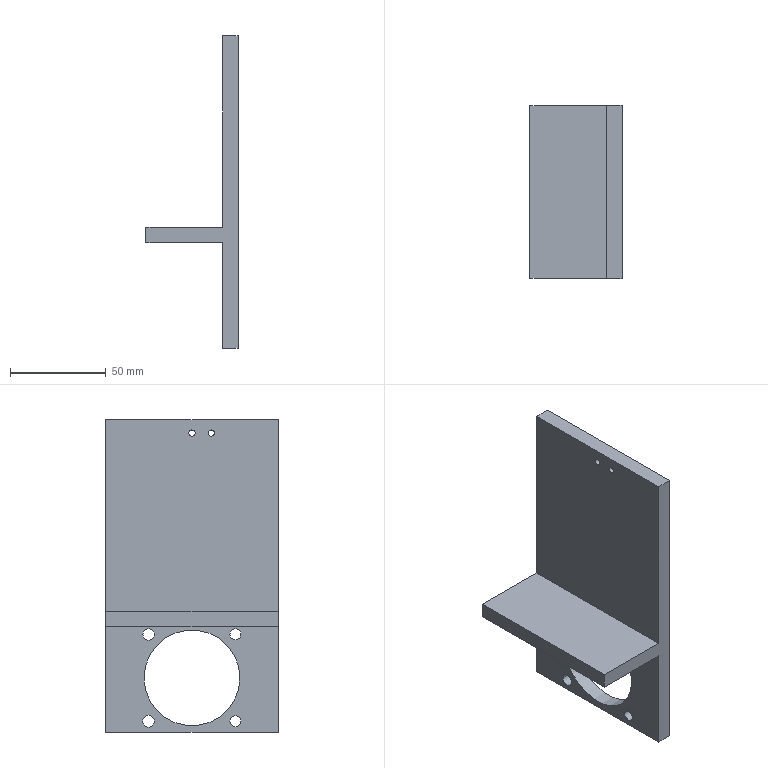Part | SolidWorks | features ICE 3, Cut 2, Extrusion 1, HoleWzd 1 | 1 solid | 24 faces | box 48 x 90 x 163 mm | volume 129456 mm3 | cylinder 14 | plane 10 | commonest cylinder face diameters 3.3 x4 5.748 x2 5.749 x2 5.963 x2 6.073 x2 49.982 x2
STEP:
#1=CARTESIAN_POINT('',(-62.,0.,99.35));
#2=VERTEX_POINT('',#1);
#3=CARTESIAN_POINT('',(-62.,0.,102.65));
#4=VERTEX_POINT('',#3);
#5=CARTESIAN_POINT('',(-62.,0.,101.));
#6=DIRECTION('',(-1.,0.,0.));
#7=DIRECTION('',(0.,-1.,0.));
#8=AXIS2_PLACEMENT_3D('',#5,#6,#7);
#9=CIRCLE('',#8,1.65);
#10=EDGE_CURVE('',#2,#4,#9,.T.);
#11=ORIENTED_EDGE('',*,*,#10,.F.);
#12=CARTESIAN_POINT('',(-70.,0.,99.35));
#13=VERTEX_POINT('',#12);
#14=CARTESIAN_POINT('',(-70.,0.,99.35));
#15=DIRECTION('',(-1.,0.,0.));
#16=VECTOR('',#15,1000.);
#17=LINE('',#14,#16);
#18=EDGE_CURVE('',#2,#13,#17,.T.);
#19=ORIENTED_EDGE('',*,*,#18,.T.);
#20=CARTESIAN_POINT('',(-70.,0.,102.65));
#21=VERTEX_POINT('',#20);
#22=CARTESIAN_POINT('',(-70.,0.,101.));
#23=DIRECTION('',(-1.,0.,0.));
#24=DIRECTION('',(0.,0.,1.));
#25=AXIS2_PLACEMENT_3D('',#22,#23,#24);
#26=CIRCLE('',#25,1.65);
#27=EDGE_CURVE('',#13,#21,#26,.T.);
#28=ORIENTED_EDGE('',*,*,#27,.T.);
#29=CARTESIAN_POINT('',(-70.,0.,102.65));
#30=DIRECTION('',(-1.,0.,0.));
#31=VECTOR('',#30,1000.);
#32=LINE('',#29,#31);
#33=EDGE_CURVE('',#4,#21,#32,.T.);
#34=ORIENTED_EDGE('',*,*,#33,.F.);
#35=EDGE_LOOP('',(#11,#19,#28,#34));
#36=FACE_OUTER_BOUND('',#35,.T.);
#37=CARTESIAN_POINT('',(-70.,0.,101.));
#38=DIRECTION('',(-1.,0.,0.));
#39=DIRECTION('',(0.,0.,1.));
#40=AXIS2_PLACEMENT_3D('',#37,#38,#39);
#41=CYLINDRICAL_SURFACE('',#40,1.65);
#42=ADVANCED_FACE('',(#36),#41,.F.);
#43=CARTESIAN_POINT('',(-62.,-10.,99.35));
#44=VERTEX_POINT('',#43);
#45=CARTESIAN_POINT('',(-62.,-10.,102.65));
#46=VERTEX_POINT('',#45);
#47=CARTESIAN_POINT('',(-62.,-10.,101.));
#48=DIRECTION('',(-1.,0.,0.));
#49=DIRECTION('',(0.,-1.,0.));
#50=AXIS2_PLACEMENT_3D('',#47,#48,#49);
#51=CIRCLE('',#50,1.65);
#52=EDGE_CURVE('',#44,#46,#51,.T.);
#53=ORIENTED_EDGE('',*,*,#52,.F.);
#54=CARTESIAN_POINT('',(-70.,-10.,99.35));
#55=VERTEX_POINT('',#54);
#56=CARTESIAN_POINT('',(-70.,-10.,99.35));
#57=DIRECTION('',(-1.,0.,0.));
#58=VECTOR('',#57,1000.);
#59=LINE('',#56,#58);
#60=EDGE_CURVE('',#44,#55,#59,.T.);
#61=ORIENTED_EDGE('',*,*,#60,.T.);
#62=CARTESIAN_POINT('',(-70.,-10.,102.65));
#63=VERTEX_POINT('',#62);
#64=CARTESIAN_POINT('',(-70.,-10.,101.));
#65=DIRECTION('',(-1.,0.,0.));
#66=DIRECTION('',(0.,0.,1.));
#67=AXIS2_PLACEMENT_3D('',#64,#65,#66);
#68=CIRCLE('',#67,1.65);
#69=EDGE_CURVE('',#55,#63,#68,.T.);
#70=ORIENTED_EDGE('',*,*,#69,.T.);
#71=CARTESIAN_POINT('',(-70.,-10.,102.65));
#72=DIRECTION('',(-1.,0.,0.));
#73=VECTOR('',#72,1000.);
#74=LINE('',#71,#73);
#75=EDGE_CURVE('',#46,#63,#74,.T.);
#76=ORIENTED_EDGE('',*,*,#75,.F.);
#77=EDGE_LOOP('',(#53,#61,#70,#76));
#78=FACE_OUTER_BOUND('',#77,.T.);
#79=CARTESIAN_POINT('',(-70.,-10.,101.));
#80=DIRECTION('',(-1.,0.,0.));
#81=DIRECTION('',(0.,0.,1.));
#82=AXIS2_PLACEMENT_3D('',#79,#80,#81);
#83=CYLINDRICAL_SURFACE('',#82,1.65);
#84=ADVANCED_FACE('',(#78),#83,.F.);
#85=CARTESIAN_POINT('',(-62.,25.609,-3.973));
#86=VERTEX_POINT('',#85);
#87=CARTESIAN_POINT('',(-62.,19.646,-3.973));
#88=VERTEX_POINT('',#87);
#89=CARTESIAN_POINT('',(-62.,22.627,-3.973));
#90=DIRECTION('',(-1.,0.,0.));
#91=DIRECTION('',(0.,-1.,0.));
#92=AXIS2_PLACEMENT_3D('',#89,#90,#91);
#93=CIRCLE('',#92,2.981);
#94=EDGE_CURVE('',#86,#88,#93,.T.);
#95=ORIENTED_EDGE('',*,*,#94,.F.);
#96=CARTESIAN_POINT('',(-70.,25.609,-3.973));
#97=VERTEX_POINT('',#96);
#98=CARTESIAN_POINT('',(-35.,25.609,-3.973));
#99=DIRECTION('',(-1.,0.,0.));
#100=VECTOR('',#99,1000.);
#101=LINE('',#98,#100);
#102=EDGE_CURVE('',#86,#97,#101,.T.);
#103=ORIENTED_EDGE('',*,*,#102,.T.);
#104=CARTESIAN_POINT('',(-70.,19.646,-3.973));
#105=VERTEX_POINT('',#104);
#106=CARTESIAN_POINT('',(-70.,22.627,-3.973));
#107=DIRECTION('',(-1.,0.,0.));
#108=DIRECTION('',(0.,-1.,0.));
#109=AXIS2_PLACEMENT_3D('',#106,#107,#108);
#110=CIRCLE('',#109,2.981);
#111=EDGE_CURVE('',#97,#105,#110,.T.);
#112=ORIENTED_EDGE('',*,*,#111,.T.);
#113=CARTESIAN_POINT('',(-35.,19.646,-3.973));
#114=DIRECTION('',(-1.,0.,0.));
#115=VECTOR('',#114,1000.);
#116=LINE('',#113,#115);
#117=EDGE_CURVE('',#88,#105,#116,.T.);
#118=ORIENTED_EDGE('',*,*,#117,.F.);
#119=EDGE_LOOP('',(#95,#103,#112,#118));
#120=FACE_OUTER_BOUND('',#119,.T.);
#121=CARTESIAN_POINT('',(-35.,22.627,-3.973));
#122=DIRECTION('',(-1.,0.,0.));
#123=DIRECTION('',(0.,-1.,0.));
#124=AXIS2_PLACEMENT_3D('',#121,#122,#123);
#125=CYLINDRICAL_SURFACE('',#124,2.981);
#126=ADVANCED_FACE('',(#120),#125,.F.);
#127=CARTESIAN_POINT('',(-62.,-19.753,-3.973));
#128=VERTEX_POINT('',#127);
#129=CARTESIAN_POINT('',(-62.,-25.502,-3.973));
#130=VERTEX_POINT('',#129);
#131=CARTESIAN_POINT('',(-62.,-22.627,-3.973));
#132=DIRECTION('',(-1.,0.,0.));
#133=DIRECTION('',(0.,-1.,0.));
#134=AXIS2_PLACEMENT_3D('',#131,#132,#133);
#135=CIRCLE('',#134,2.874);
#136=EDGE_CURVE('',#128,#130,#135,.T.);
#137=ORIENTED_EDGE('',*,*,#136,.F.);
#138=CARTESIAN_POINT('',(-70.,-19.753,-3.973));
#139=VERTEX_POINT('',#138);
#140=CARTESIAN_POINT('',(-35.,-19.753,-3.973));
#141=DIRECTION('',(-1.,0.,0.));
#142=VECTOR('',#141,1000.);
#143=LINE('',#140,#142);
#144=EDGE_CURVE('',#128,#139,#143,.T.);
#145=ORIENTED_EDGE('',*,*,#144,.T.);
#146=CARTESIAN_POINT('',(-70.,-25.502,-3.973));
#147=VERTEX_POINT('',#146);
#148=CARTESIAN_POINT('',(-70.,-22.627,-3.973));
#149=DIRECTION('',(-1.,0.,0.));
#150=DIRECTION('',(0.,-1.,0.));
#151=AXIS2_PLACEMENT_3D('',#148,#149,#150);
#152=CIRCLE('',#151,2.874);
#153=EDGE_CURVE('',#139,#147,#152,.T.);
#154=ORIENTED_EDGE('',*,*,#153,.T.);
#155=CARTESIAN_POINT('',(-35.,-25.502,-3.973));
#156=DIRECTION('',(-1.,0.,0.));
#157=VECTOR('',#156,1000.);
#158=LINE('',#155,#157);
#159=EDGE_CURVE('',#130,#147,#158,.T.);
#160=ORIENTED_EDGE('',*,*,#159,.F.);
#161=EDGE_LOOP('',(#137,#145,#154,#160));
#162=FACE_OUTER_BOUND('',#161,.T.);
#163=CARTESIAN_POINT('',(-35.,-22.627,-3.973));
#164=DIRECTION('',(-1.,0.,0.));
#165=DIRECTION('',(0.,-1.,0.));
#166=AXIS2_PLACEMENT_3D('',#163,#164,#165);
#167=CYLINDRICAL_SURFACE('',#166,2.874);
#168=ADVANCED_FACE('',(#162),#167,.F.);
#169=CARTESIAN_POINT('',(-62.,-19.754,-49.227));
#170=VERTEX_POINT('',#169);
#171=CARTESIAN_POINT('',(-62.,-25.501,-49.227));
#172=VERTEX_POINT('',#171);
#173=CARTESIAN_POINT('',(-62.,-22.627,-49.227));
#174=DIRECTION('',(-1.,0.,0.));
#175=DIRECTION('',(0.,-1.,0.));
#176=AXIS2_PLACEMENT_3D('',#173,#174,#175);
#177=CIRCLE('',#176,2.874);
#178=EDGE_CURVE('',#170,#172,#177,.T.);
#179=ORIENTED_EDGE('',*,*,#178,.F.);
#180=CARTESIAN_POINT('',(-70.,-19.754,-49.227));
#181=VERTEX_POINT('',#180);
#182=CARTESIAN_POINT('',(-35.,-19.754,-49.227));
#183=DIRECTION('',(-1.,0.,0.));
#184=VECTOR('',#183,1000.);
#185=LINE('',#182,#184);
#186=EDGE_CURVE('',#170,#181,#185,.T.);
#187=ORIENTED_EDGE('',*,*,#186,.T.);
#188=CARTESIAN_POINT('',(-70.,-25.501,-49.227));
#189=VERTEX_POINT('',#188);
#190=CARTESIAN_POINT('',(-70.,-22.627,-49.227));
#191=DIRECTION('',(-1.,0.,0.));
#192=DIRECTION('',(0.,-1.,0.));
#193=AXIS2_PLACEMENT_3D('',#190,#191,#192);
#194=CIRCLE('',#193,2.874);
#195=EDGE_CURVE('',#181,#189,#194,.T.);
#196=ORIENTED_EDGE('',*,*,#195,.T.);
#197=CARTESIAN_POINT('',(-35.,-25.501,-49.227));
#198=DIRECTION('',(-1.,0.,0.));
#199=VECTOR('',#198,1000.);
#200=LINE('',#197,#199);
#201=EDGE_CURVE('',#172,#189,#200,.T.);
#202=ORIENTED_EDGE('',*,*,#201,.F.);
#203=EDGE_LOOP('',(#179,#187,#196,#202));
#204=FACE_OUTER_BOUND('',#203,.T.);
#205=CARTESIAN_POINT('',(-35.,-22.627,-49.227));
#206=DIRECTION('',(-1.,0.,0.));
#207=DIRECTION('',(0.,-1.,0.));
#208=AXIS2_PLACEMENT_3D('',#205,#206,#207);
#209=CYLINDRICAL_SURFACE('',#208,2.874);
#210=ADVANCED_FACE('',(#204),#209,.F.);
#211=CARTESIAN_POINT('',(-62.,25.664,-49.227));
#212=VERTEX_POINT('',#211);
#213=CARTESIAN_POINT('',(-62.,19.591,-49.227));
#214=VERTEX_POINT('',#213);
#215=CARTESIAN_POINT('',(-62.,22.627,-49.227));
#216=DIRECTION('',(-1.,0.,0.));
#217=DIRECTION('',(0.,-1.,0.));
#218=AXIS2_PLACEMENT_3D('',#215,#216,#217);
#219=CIRCLE('',#218,3.036);
#220=EDGE_CURVE('',#212,#214,#219,.T.);
#221=ORIENTED_EDGE('',*,*,#220,.F.);
#222=CARTESIAN_POINT('',(-70.,25.664,-49.227));
#223=VERTEX_POINT('',#222);
#224=CARTESIAN_POINT('',(-35.,25.664,-49.227));
#225=DIRECTION('',(-1.,0.,0.));
#226=VECTOR('',#225,1000.);
#227=LINE('',#224,#226);
#228=EDGE_CURVE('',#212,#223,#227,.T.);
#229=ORIENTED_EDGE('',*,*,#228,.T.);
#230=CARTESIAN_POINT('',(-70.,19.591,-49.227));
#231=VERTEX_POINT('',#230);
#232=CARTESIAN_POINT('',(-70.,22.627,-49.227));
#233=DIRECTION('',(-1.,0.,0.));
#234=DIRECTION('',(0.,-1.,0.));
#235=AXIS2_PLACEMENT_3D('',#232,#233,#234);
#236=CIRCLE('',#235,3.036);
#237=EDGE_CURVE('',#223,#231,#236,.T.);
#238=ORIENTED_EDGE('',*,*,#237,.T.);
#239=CARTESIAN_POINT('',(-35.,19.591,-49.227));
#240=DIRECTION('',(-1.,0.,0.));
#241=VECTOR('',#240,1000.);
#242=LINE('',#239,#241);
#243=EDGE_CURVE('',#214,#231,#242,.T.);
#244=ORIENTED_EDGE('',*,*,#243,.F.);
#245=EDGE_LOOP('',(#221,#229,#238,#244));
#246=FACE_OUTER_BOUND('',#245,.T.);
#247=CARTESIAN_POINT('',(-35.,22.627,-49.227));
#248=DIRECTION('',(-1.,0.,0.));
#249=DIRECTION('',(0.,-1.,0.));
#250=AXIS2_PLACEMENT_3D('',#247,#248,#249);
#251=CYLINDRICAL_SURFACE('',#250,3.036);
#252=ADVANCED_FACE('',(#246),#251,.F.);
#253=CARTESIAN_POINT('',(-62.,25.,-26.6));
#254=VERTEX_POINT('',#253);
#255=CARTESIAN_POINT('',(-62.,-24.982,-26.6));
#256=VERTEX_POINT('',#255);
#257=CARTESIAN_POINT('',(-62.,0.009138,-26.6));
#258=DIRECTION('',(-1.,0.,0.));
#259=DIRECTION('',(0.,-1.,0.));
#260=AXIS2_PLACEMENT_3D('',#257,#258,#259);
#261=CIRCLE('',#260,24.991);
#262=EDGE_CURVE('',#254,#256,#261,.T.);
#263=ORIENTED_EDGE('',*,*,#262,.F.);
#264=CARTESIAN_POINT('',(-70.,25.,-26.6));
#265=VERTEX_POINT('',#264);
#266=CARTESIAN_POINT('',(-35.,25.,-26.6));
#267=DIRECTION('',(-1.,0.,0.));
#268=VECTOR('',#267,1000.);
#269=LINE('',#266,#268);
#270=EDGE_CURVE('',#254,#265,#269,.T.);
#271=ORIENTED_EDGE('',*,*,#270,.T.);
#272=CARTESIAN_POINT('',(-70.,-24.982,-26.6));
#273=VERTEX_POINT('',#272);
#274=CARTESIAN_POINT('',(-70.,0.009138,-26.6));
#275=DIRECTION('',(-1.,0.,0.));
#276=DIRECTION('',(0.,-1.,0.));
#277=AXIS2_PLACEMENT_3D('',#274,#275,#276);
#278=CIRCLE('',#277,24.991);
#279=EDGE_CURVE('',#265,#273,#278,.T.);
#280=ORIENTED_EDGE('',*,*,#279,.T.);
#281=CARTESIAN_POINT('',(-35.,-24.982,-26.6));
#282=DIRECTION('',(-1.,0.,0.));
#283=VECTOR('',#282,1000.);
#284=LINE('',#281,#283);
#285=EDGE_CURVE('',#256,#273,#284,.T.);
#286=ORIENTED_EDGE('',*,*,#285,.F.);
#287=EDGE_LOOP('',(#263,#271,#280,#286));
#288=FACE_OUTER_BOUND('',#287,.T.);
#289=CARTESIAN_POINT('',(-35.,0.009138,-26.6));
#290=DIRECTION('',(-1.,0.,0.));
#291=DIRECTION('',(0.,-1.,0.));
#292=AXIS2_PLACEMENT_3D('',#289,#290,#291);
#293=CYLINDRICAL_SURFACE('',#292,24.991);
#294=ADVANCED_FACE('',(#288),#293,.F.);
#295=CARTESIAN_POINT('',(-70.,-45.,0.));
#296=VERTEX_POINT('',#295);
#297=CARTESIAN_POINT('',(-70.,45.,0.));
#298=VERTEX_POINT('',#297);
#299=CARTESIAN_POINT('',(-70.,-45.,0.));
#300=DIRECTION('',(0.,1.,0.));
#301=VECTOR('',#300,1000.);
#302=LINE('',#299,#301);
#303=EDGE_CURVE('',#296,#298,#302,.T.);
#304=ORIENTED_EDGE('',*,*,#303,.F.);
#305=CARTESIAN_POINT('',(-110.,-45.,0.));
#306=VERTEX_POINT('',#305);
#307=CARTESIAN_POINT('',(-60.,-45.,0.));
#308=DIRECTION('',(1.,0.,0.));
#309=VECTOR('',#308,1000.);
#310=LINE('',#307,#309);
#311=EDGE_CURVE('',#306,#296,#310,.T.);
#312=ORIENTED_EDGE('',*,*,#311,.F.);
#313=CARTESIAN_POINT('',(-110.,45.,0.));
#314=VERTEX_POINT('',#313);
#315=CARTESIAN_POINT('',(-110.,45.,0.));
#316=DIRECTION('',(0.,-1.,0.));
#317=VECTOR('',#316,1000.);
#318=LINE('',#315,#317);
#319=EDGE_CURVE('',#314,#306,#318,.T.);
#320=ORIENTED_EDGE('',*,*,#319,.F.);
#321=CARTESIAN_POINT('',(-60.,45.,0.));
#322=DIRECTION('',(-1.,0.,0.));
#323=VECTOR('',#322,1000.);
#324=LINE('',#321,#323);
#325=EDGE_CURVE('',#298,#314,#324,.T.);
#326=ORIENTED_EDGE('',*,*,#325,.F.);
#327=EDGE_LOOP('',(#304,#312,#320,#326));
#328=FACE_OUTER_BOUND('',#327,.T.);
#329=CARTESIAN_POINT('',(0.,0.,0.));
#330=DIRECTION('',(0.,0.,1.));
#331=DIRECTION('',(1.,0.,0.));
#332=AXIS2_PLACEMENT_3D('',#329,#330,#331);
#333=PLANE('',#332);
#334=ADVANCED_FACE('',(#328),#333,.F.);
#335=CARTESIAN_POINT('',(-70.,45.,8.));
#336=VERTEX_POINT('',#335);
#337=CARTESIAN_POINT('',(-70.,-45.,8.));
#338=VERTEX_POINT('',#337);
#339=CARTESIAN_POINT('',(-70.,45.,8.));
#340=DIRECTION('',(0.,-1.,0.));
#341=VECTOR('',#340,1000.);
#342=LINE('',#339,#341);
#343=EDGE_CURVE('',#336,#338,#342,.T.);
#344=ORIENTED_EDGE('',*,*,#343,.F.);
#345=CARTESIAN_POINT('',(-110.,45.,8.));
#346=VERTEX_POINT('',#345);
#347=CARTESIAN_POINT('',(-60.,45.,8.));
#348=DIRECTION('',(-1.,0.,0.));
#349=VECTOR('',#348,1000.);
#350=LINE('',#347,#349);
#351=EDGE_CURVE('',#336,#346,#350,.T.);
#352=ORIENTED_EDGE('',*,*,#351,.T.);
#353=CARTESIAN_POINT('',(-110.,-45.,8.));
#354=VERTEX_POINT('',#353);
#355=CARTESIAN_POINT('',(-110.,-45.,8.));
#356=DIRECTION('',(0.,1.,0.));
#357=VECTOR('',#356,1000.);
#358=LINE('',#355,#357);
#359=EDGE_CURVE('',#354,#346,#358,.T.);
#360=ORIENTED_EDGE('',*,*,#359,.F.);
#361=CARTESIAN_POINT('',(-60.,-45.,8.));
#362=DIRECTION('',(1.,0.,0.));
#363=VECTOR('',#362,1000.);
#364=LINE('',#361,#363);
#365=EDGE_CURVE('',#354,#338,#364,.T.);
#366=ORIENTED_EDGE('',*,*,#365,.T.);
#367=EDGE_LOOP('',(#344,#352,#360,#366));
#368=FACE_OUTER_BOUND('',#367,.T.);
#369=CARTESIAN_POINT('',(0.,0.,8.));
#370=DIRECTION('',(0.,0.,1.));
#371=DIRECTION('',(1.,0.,0.));
#372=AXIS2_PLACEMENT_3D('',#369,#370,#371);
#373=PLANE('',#372);
#374=ADVANCED_FACE('',(#368),#373,.T.);
#375=CARTESIAN_POINT('',(-62.,45.,108.));
#376=VERTEX_POINT('',#375);
#377=CARTESIAN_POINT('',(-62.,45.,-55.));
#378=VERTEX_POINT('',#377);
#379=CARTESIAN_POINT('',(-62.,45.,108.));
#380=DIRECTION('',(0.,0.,-1.));
#381=VECTOR('',#380,1000.);
#382=LINE('',#379,#381);
#383=EDGE_CURVE('',#376,#378,#382,.T.);
#384=ORIENTED_EDGE('',*,*,#383,.T.);
#385=CARTESIAN_POINT('',(-70.,45.,-55.));
#386=VERTEX_POINT('',#385);
#387=CARTESIAN_POINT('',(-70.,45.,-55.));
#388=DIRECTION('',(1.,0.,0.));
#389=VECTOR('',#388,1000.);
#390=LINE('',#387,#389);
#391=EDGE_CURVE('',#386,#378,#390,.T.);
#392=ORIENTED_EDGE('',*,*,#391,.F.);
#393=CARTESIAN_POINT('',(-70.,45.,-55.));
#394=DIRECTION('',(0.,0.,1.));
#395=VECTOR('',#394,1000.);
#396=LINE('',#393,#395);
#397=EDGE_CURVE('',#386,#298,#396,.T.);
#398=ORIENTED_EDGE('',*,*,#397,.T.);
#399=ORIENTED_EDGE('',*,*,#325,.T.);
#400=CARTESIAN_POINT('',(-110.,45.,8.));
#401=DIRECTION('',(0.,0.,-1.));
#402=VECTOR('',#401,1000.);
#403=LINE('',#400,#402);
#404=EDGE_CURVE('',#346,#314,#403,.T.);
#405=ORIENTED_EDGE('',*,*,#404,.F.);
#406=ORIENTED_EDGE('',*,*,#351,.F.);
#407=CARTESIAN_POINT('',(-70.,45.,108.));
#408=VERTEX_POINT('',#407);
#409=CARTESIAN_POINT('',(-70.,45.,108.));
#410=DIRECTION('',(0.,0.,-1.));
#411=VECTOR('',#410,1000.);
#412=LINE('',#409,#411);
#413=EDGE_CURVE('',#408,#336,#412,.T.);
#414=ORIENTED_EDGE('',*,*,#413,.F.);
#415=CARTESIAN_POINT('',(-70.,45.,108.));
#416=DIRECTION('',(-1.,0.,0.));
#417=VECTOR('',#416,1000.);
#418=LINE('',#415,#417);
#419=EDGE_CURVE('',#376,#408,#418,.T.);
#420=ORIENTED_EDGE('',*,*,#419,.F.);
#421=EDGE_LOOP('',(#384,#392,#398,#399,#405,#406,#414,#420));
#422=FACE_OUTER_BOUND('',#421,.T.);
#423=CARTESIAN_POINT('',(-60.,45.,8.));
#424=DIRECTION('',(0.,-1.,0.));
#425=DIRECTION('',(0.,0.,-1.));
#426=AXIS2_PLACEMENT_3D('',#423,#424,#425);
#427=PLANE('',#426);
#428=ADVANCED_FACE('',(#422),#427,.F.);
#429=ORIENTED_EDGE('',*,*,#311,.T.);
#430=CARTESIAN_POINT('',(-70.,-45.,-55.));
#431=VERTEX_POINT('',#430);
#432=CARTESIAN_POINT('',(-70.,-45.,-55.));
#433=DIRECTION('',(0.,0.,1.));
#434=VECTOR('',#433,1000.);
#435=LINE('',#432,#434);
#436=EDGE_CURVE('',#431,#296,#435,.T.);
#437=ORIENTED_EDGE('',*,*,#436,.F.);
#438=CARTESIAN_POINT('',(-62.,-45.,-55.));
#439=VERTEX_POINT('',#438);
#440=CARTESIAN_POINT('',(-62.,-45.,-55.));
#441=DIRECTION('',(-1.,0.,0.));
#442=VECTOR('',#441,1000.);
#443=LINE('',#440,#442);
#444=EDGE_CURVE('',#439,#431,#443,.T.);
#445=ORIENTED_EDGE('',*,*,#444,.F.);
#446=CARTESIAN_POINT('',(-62.,-45.,108.));
#447=VERTEX_POINT('',#446);
#448=CARTESIAN_POINT('',(-62.,-45.,108.));
#449=DIRECTION('',(0.,0.,-1.));
#450=VECTOR('',#449,1000.);
#451=LINE('',#448,#450);
#452=EDGE_CURVE('',#447,#439,#451,.T.);
#453=ORIENTED_EDGE('',*,*,#452,.F.);
#454=CARTESIAN_POINT('',(-70.,-45.,108.));
#455=VERTEX_POINT('',#454);
#456=CARTESIAN_POINT('',(-70.,-45.,108.));
#457=DIRECTION('',(1.,0.,0.));
#458=VECTOR('',#457,1000.);
#459=LINE('',#456,#458);
#460=EDGE_CURVE('',#455,#447,#459,.T.);
#461=ORIENTED_EDGE('',*,*,#460,.F.);
#462=CARTESIAN_POINT('',(-70.,-45.,108.));
#463=DIRECTION('',(0.,0.,-1.));
#464=VECTOR('',#463,1000.);
#465=LINE('',#462,#464);
#466=EDGE_CURVE('',#455,#338,#465,.T.);
#467=ORIENTED_EDGE('',*,*,#466,.T.);
#468=ORIENTED_EDGE('',*,*,#365,.F.);
#469=CARTESIAN_POINT('',(-110.,-45.,0.));
#470=DIRECTION('',(0.,0.,1.));
#471=VECTOR('',#470,1000.);
#472=LINE('',#469,#471);
#473=EDGE_CURVE('',#306,#354,#472,.T.);
#474=ORIENTED_EDGE('',*,*,#473,.F.);
#475=EDGE_LOOP('',(#429,#437,#445,#453,#461,#467,#468,#474));
#476=FACE_OUTER_BOUND('',#475,.T.);
#477=CARTESIAN_POINT('',(-60.,-45.,8.));
#478=DIRECTION('',(0.,1.,0.));
#479=DIRECTION('',(0.,0.,1.));
#480=AXIS2_PLACEMENT_3D('',#477,#478,#479);
#481=PLANE('',#480);
#482=ADVANCED_FACE('',(#476),#481,.F.);
#483=ORIENTED_EDGE('',*,*,#404,.T.);
#484=ORIENTED_EDGE('',*,*,#319,.T.);
#485=ORIENTED_EDGE('',*,*,#473,.T.);
#486=ORIENTED_EDGE('',*,*,#359,.T.);
#487=EDGE_LOOP('',(#483,#484,#485,#486));
#488=FACE_OUTER_BOUND('',#487,.T.);
#489=CARTESIAN_POINT('',(-110.,0.,0.));
#490=DIRECTION('',(-1.,0.,0.));
#491=DIRECTION('',(0.,-1.,0.));
#492=AXIS2_PLACEMENT_3D('',#489,#490,#491);
#493=PLANE('',#492);
#494=ADVANCED_FACE('',(#488),#493,.T.);
#495=CARTESIAN_POINT('',(-70.,0.,101.));
#496=DIRECTION('',(-1.,0.,0.));
#497=DIRECTION('',(0.,0.,1.));
#498=AXIS2_PLACEMENT_3D('',#495,#496,#497);
#499=CIRCLE('',#498,1.65);
#500=EDGE_CURVE('',#21,#13,#499,.T.);
#501=ORIENTED_EDGE('',*,*,#500,.F.);
#502=ORIENTED_EDGE('',*,*,#27,.F.);
#503=EDGE_LOOP('',(#501,#502));
#504=FACE_BOUND('',#503,.T.);
#505=CARTESIAN_POINT('',(-70.,-10.,101.));
#506=DIRECTION('',(-1.,0.,0.));
#507=DIRECTION('',(0.,0.,1.));
#508=AXIS2_PLACEMENT_3D('',#505,#506,#507);
#509=CIRCLE('',#508,1.65);
#510=EDGE_CURVE('',#63,#55,#509,.T.);
#511=ORIENTED_EDGE('',*,*,#510,.F.);
#512=ORIENTED_EDGE('',*,*,#69,.F.);
#513=EDGE_LOOP('',(#511,#512));
#514=FACE_BOUND('',#513,.T.);
#515=ORIENTED_EDGE('',*,*,#343,.T.);
#516=ORIENTED_EDGE('',*,*,#466,.F.);
#517=CARTESIAN_POINT('',(-70.,45.,108.));
#518=DIRECTION('',(0.,-1.,0.));
#519=VECTOR('',#518,1000.);
#520=LINE('',#517,#519);
#521=EDGE_CURVE('',#408,#455,#520,.T.);
#522=ORIENTED_EDGE('',*,*,#521,.F.);
#523=ORIENTED_EDGE('',*,*,#413,.T.);
#524=EDGE_LOOP('',(#515,#516,#522,#523));
#525=FACE_OUTER_BOUND('',#524,.T.);
#526=CARTESIAN_POINT('',(-70.,45.,108.));
#527=DIRECTION('',(1.,0.,0.));
#528=DIRECTION('',(0.,1.,0.));
#529=AXIS2_PLACEMENT_3D('',#526,#527,#528);
#530=PLANE('',#529);
#531=ADVANCED_FACE('',(#504,#514,#525),#530,.F.);
#532=CARTESIAN_POINT('',(-62.,0.,101.));
#533=DIRECTION('',(-1.,0.,0.));
#534=DIRECTION('',(0.,-1.,0.));
#535=AXIS2_PLACEMENT_3D('',#532,#533,#534);
#536=CIRCLE('',#535,1.65);
#537=EDGE_CURVE('',#4,#2,#536,.T.);
#538=ORIENTED_EDGE('',*,*,#537,.T.);
#539=ORIENTED_EDGE('',*,*,#10,.T.);
#540=EDGE_LOOP('',(#538,#539));
#541=FACE_BOUND('',#540,.T.);
#542=CARTESIAN_POINT('',(-62.,-10.,101.));
#543=DIRECTION('',(-1.,0.,0.));
#544=DIRECTION('',(0.,-1.,0.));
#545=AXIS2_PLACEMENT_3D('',#542,#543,#544);
#546=CIRCLE('',#545,1.65);
#547=EDGE_CURVE('',#46,#44,#546,.T.);
#548=ORIENTED_EDGE('',*,*,#547,.T.);
#549=ORIENTED_EDGE('',*,*,#52,.T.);
#550=EDGE_LOOP('',(#548,#549));
#551=FACE_BOUND('',#550,.T.);
#552=CARTESIAN_POINT('',(-62.,22.627,-3.973));
#553=DIRECTION('',(-1.,0.,0.));
#554=DIRECTION('',(0.,-1.,0.));
#555=AXIS2_PLACEMENT_3D('',#552,#553,#554);
#556=CIRCLE('',#555,2.981);
#557=EDGE_CURVE('',#88,#86,#556,.T.);
#558=ORIENTED_EDGE('',*,*,#557,.T.);
#559=ORIENTED_EDGE('',*,*,#94,.T.);
#560=EDGE_LOOP('',(#558,#559));
#561=FACE_BOUND('',#560,.T.);
#562=CARTESIAN_POINT('',(-62.,-22.627,-3.973));
#563=DIRECTION('',(-1.,0.,0.));
#564=DIRECTION('',(0.,-1.,0.));
#565=AXIS2_PLACEMENT_3D('',#562,#563,#564);
#566=CIRCLE('',#565,2.874);
#567=EDGE_CURVE('',#130,#128,#566,.T.);
#568=ORIENTED_EDGE('',*,*,#567,.T.);
#569=ORIENTED_EDGE('',*,*,#136,.T.);
#570=EDGE_LOOP('',(#568,#569));
#571=FACE_BOUND('',#570,.T.);
#572=CARTESIAN_POINT('',(-62.,-22.627,-49.227));
#573=DIRECTION('',(-1.,0.,0.));
#574=DIRECTION('',(0.,-1.,0.));
#575=AXIS2_PLACEMENT_3D('',#572,#573,#574);
#576=CIRCLE('',#575,2.874);
#577=EDGE_CURVE('',#172,#170,#576,.T.);
#578=ORIENTED_EDGE('',*,*,#577,.T.);
#579=ORIENTED_EDGE('',*,*,#178,.T.);
#580=EDGE_LOOP('',(#578,#579));
#581=FACE_BOUND('',#580,.T.);
#582=CARTESIAN_POINT('',(-62.,22.627,-49.227));
#583=DIRECTION('',(-1.,0.,0.));
#584=DIRECTION('',(0.,-1.,0.));
#585=AXIS2_PLACEMENT_3D('',#582,#583,#584);
#586=CIRCLE('',#585,3.036);
#587=EDGE_CURVE('',#214,#212,#586,.T.);
#588=ORIENTED_EDGE('',*,*,#587,.T.);
#589=ORIENTED_EDGE('',*,*,#220,.T.);
#590=EDGE_LOOP('',(#588,#589));
#591=FACE_BOUND('',#590,.T.);
#592=CARTESIAN_POINT('',(-62.,0.009138,-26.6));
#593=DIRECTION('',(-1.,0.,0.));
#594=DIRECTION('',(0.,-1.,0.));
#595=AXIS2_PLACEMENT_3D('',#592,#593,#594);
#596=CIRCLE('',#595,24.991);
#597=EDGE_CURVE('',#256,#254,#596,.T.);
#598=ORIENTED_EDGE('',*,*,#597,.T.);
#599=ORIENTED_EDGE('',*,*,#262,.T.);
#600=EDGE_LOOP('',(#598,#599));
#601=FACE_BOUND('',#600,.T.);
#602=ORIENTED_EDGE('',*,*,#452,.T.);
#603=CARTESIAN_POINT('',(-62.,45.,-55.));
#604=DIRECTION('',(0.,-1.,0.));
#605=VECTOR('',#604,1000.);
#606=LINE('',#603,#605);
#607=EDGE_CURVE('',#378,#439,#606,.T.);
#608=ORIENTED_EDGE('',*,*,#607,.F.);
#609=ORIENTED_EDGE('',*,*,#383,.F.);
#610=CARTESIAN_POINT('',(-62.,45.,108.));
#611=DIRECTION('',(0.,1.,0.));
#612=VECTOR('',#611,1000.);
#613=LINE('',#610,#612);
#614=EDGE_CURVE('',#447,#376,#613,.T.);
#615=ORIENTED_EDGE('',*,*,#614,.F.);
#616=EDGE_LOOP('',(#602,#608,#609,#615));
#617=FACE_OUTER_BOUND('',#616,.T.);
#618=CARTESIAN_POINT('',(-62.,45.,108.));
#619=DIRECTION('',(-1.,0.,0.));
#620=DIRECTION('',(0.,-1.,0.));
#621=AXIS2_PLACEMENT_3D('',#618,#619,#620);
#622=PLANE('',#621);
#623=ADVANCED_FACE('',(#541,#551,#561,#571,#581,#591,#601,#617),#622,.F.);
#624=ORIENTED_EDGE('',*,*,#521,.T.);
#625=ORIENTED_EDGE('',*,*,#460,.T.);
#626=ORIENTED_EDGE('',*,*,#614,.T.);
#627=ORIENTED_EDGE('',*,*,#419,.T.);
#628=EDGE_LOOP('',(#624,#625,#626,#627));
#629=FACE_OUTER_BOUND('',#628,.T.);
#630=CARTESIAN_POINT('',(0.,0.,108.));
#631=DIRECTION('',(0.,0.,1.));
#632=DIRECTION('',(1.,0.,0.));
#633=AXIS2_PLACEMENT_3D('',#630,#631,#632);
#634=PLANE('',#633);
#635=ADVANCED_FACE('',(#629),#634,.T.);
#636=CARTESIAN_POINT('',(-70.,22.627,-3.973));
#637=DIRECTION('',(-1.,0.,0.));
#638=DIRECTION('',(0.,-1.,0.));
#639=AXIS2_PLACEMENT_3D('',#636,#637,#638);
#640=CIRCLE('',#639,2.981);
#641=EDGE_CURVE('',#105,#97,#640,.T.);
#642=ORIENTED_EDGE('',*,*,#641,.F.);
#643=ORIENTED_EDGE('',*,*,#111,.F.);
#644=EDGE_LOOP('',(#642,#643));
#645=FACE_BOUND('',#644,.T.);
#646=CARTESIAN_POINT('',(-70.,-22.627,-3.973));
#647=DIRECTION('',(-1.,0.,0.));
#648=DIRECTION('',(0.,-1.,0.));
#649=AXIS2_PLACEMENT_3D('',#646,#647,#648);
#650=CIRCLE('',#649,2.874);
#651=EDGE_CURVE('',#147,#139,#650,.T.);
#652=ORIENTED_EDGE('',*,*,#651,.F.);
#653=ORIENTED_EDGE('',*,*,#153,.F.);
#654=EDGE_LOOP('',(#652,#653));
#655=FACE_BOUND('',#654,.T.);
#656=CARTESIAN_POINT('',(-70.,-22.627,-49.227));
#657=DIRECTION('',(-1.,0.,0.));
#658=DIRECTION('',(0.,-1.,0.));
#659=AXIS2_PLACEMENT_3D('',#656,#657,#658);
#660=CIRCLE('',#659,2.874);
#661=EDGE_CURVE('',#189,#181,#660,.T.);
#662=ORIENTED_EDGE('',*,*,#661,.F.);
#663=ORIENTED_EDGE('',*,*,#195,.F.);
#664=EDGE_LOOP('',(#662,#663));
#665=FACE_BOUND('',#664,.T.);
#666=CARTESIAN_POINT('',(-70.,22.627,-49.227));
#667=DIRECTION('',(-1.,0.,0.));
#668=DIRECTION('',(0.,-1.,0.));
#669=AXIS2_PLACEMENT_3D('',#666,#667,#668);
#670=CIRCLE('',#669,3.036);
#671=EDGE_CURVE('',#231,#223,#670,.T.);
#672=ORIENTED_EDGE('',*,*,#671,.F.);
#673=ORIENTED_EDGE('',*,*,#237,.F.);
#674=EDGE_LOOP('',(#672,#673));
#675=FACE_BOUND('',#674,.T.);
#676=CARTESIAN_POINT('',(-70.,0.009138,-26.6));
#677=DIRECTION('',(-1.,0.,0.));
#678=DIRECTION('',(0.,-1.,0.));
#679=AXIS2_PLACEMENT_3D('',#676,#677,#678);
#680=CIRCLE('',#679,24.991);
#681=EDGE_CURVE('',#273,#265,#680,.T.);
#682=ORIENTED_EDGE('',*,*,#681,.F.);
#683=ORIENTED_EDGE('',*,*,#279,.F.);
#684=EDGE_LOOP('',(#682,#683));
#685=FACE_BOUND('',#684,.T.);
#686=ORIENTED_EDGE('',*,*,#303,.T.);
#687=ORIENTED_EDGE('',*,*,#397,.F.);
#688=CARTESIAN_POINT('',(-70.,-45.,-55.));
#689=DIRECTION('',(0.,1.,0.));
#690=VECTOR('',#689,1000.);
#691=LINE('',#688,#690);
#692=EDGE_CURVE('',#431,#386,#691,.T.);
#693=ORIENTED_EDGE('',*,*,#692,.F.);
#694=ORIENTED_EDGE('',*,*,#436,.T.);
#695=EDGE_LOOP('',(#686,#687,#693,#694));
#696=FACE_OUTER_BOUND('',#695,.T.);
#697=CARTESIAN_POINT('',(-70.,-45.,-55.));
#698=DIRECTION('',(1.,0.,0.));
#699=DIRECTION('',(0.,1.,0.));
#700=AXIS2_PLACEMENT_3D('',#697,#698,#699);
#701=PLANE('',#700);
#702=ADVANCED_FACE('',(#645,#655,#665,#675,#685,#696),#701,.F.);
#703=ORIENTED_EDGE('',*,*,#391,.T.);
#704=ORIENTED_EDGE('',*,*,#607,.T.);
#705=ORIENTED_EDGE('',*,*,#444,.T.);
#706=ORIENTED_EDGE('',*,*,#692,.T.);
#707=EDGE_LOOP('',(#703,#704,#705,#706));
#708=FACE_OUTER_BOUND('',#707,.T.);
#709=CARTESIAN_POINT('',(0.,0.,-55.));
#710=DIRECTION('',(0.,0.,-1.));
#711=DIRECTION('',(-1.,0.,0.));
#712=AXIS2_PLACEMENT_3D('',#709,#710,#711);
#713=PLANE('',#712);
#714=ADVANCED_FACE('',(#708),#713,.T.);
#715=ORIENTED_EDGE('',*,*,#270,.F.);
#716=ORIENTED_EDGE('',*,*,#597,.F.);
#717=ORIENTED_EDGE('',*,*,#285,.T.);
#718=ORIENTED_EDGE('',*,*,#681,.T.);
#719=EDGE_LOOP('',(#715,#716,#717,#718));
#720=FACE_OUTER_BOUND('',#719,.T.);
#721=CARTESIAN_POINT('',(-35.,0.009138,-26.6));
#722=DIRECTION('',(-1.,0.,0.));
#723=DIRECTION('',(0.,-1.,0.));
#724=AXIS2_PLACEMENT_3D('',#721,#722,#723);
#725=CYLINDRICAL_SURFACE('',#724,24.991);
#726=ADVANCED_FACE('',(#720),#725,.F.);
#727=ORIENTED_EDGE('',*,*,#228,.F.);
#728=ORIENTED_EDGE('',*,*,#587,.F.);
#729=ORIENTED_EDGE('',*,*,#243,.T.);
#730=ORIENTED_EDGE('',*,*,#671,.T.);
#731=EDGE_LOOP('',(#727,#728,#729,#730));
#732=FACE_OUTER_BOUND('',#731,.T.);
#733=CARTESIAN_POINT('',(-35.,22.627,-49.227));
#734=DIRECTION('',(-1.,0.,0.));
#735=DIRECTION('',(0.,-1.,0.));
#736=AXIS2_PLACEMENT_3D('',#733,#734,#735);
#737=CYLINDRICAL_SURFACE('',#736,3.036);
#738=ADVANCED_FACE('',(#732),#737,.F.);
#739=ORIENTED_EDGE('',*,*,#186,.F.);
#740=ORIENTED_EDGE('',*,*,#577,.F.);
#741=ORIENTED_EDGE('',*,*,#201,.T.);
#742=ORIENTED_EDGE('',*,*,#661,.T.);
#743=EDGE_LOOP('',(#739,#740,#741,#742));
#744=FACE_OUTER_BOUND('',#743,.T.);
#745=CARTESIAN_POINT('',(-35.,-22.627,-49.227));
#746=DIRECTION('',(-1.,0.,0.));
#747=DIRECTION('',(0.,-1.,0.));
#748=AXIS2_PLACEMENT_3D('',#745,#746,#747);
#749=CYLINDRICAL_SURFACE('',#748,2.874);
#750=ADVANCED_FACE('',(#744),#749,.F.);
#751=ORIENTED_EDGE('',*,*,#144,.F.);
#752=ORIENTED_EDGE('',*,*,#567,.F.);
#753=ORIENTED_EDGE('',*,*,#159,.T.);
#754=ORIENTED_EDGE('',*,*,#651,.T.);
#755=EDGE_LOOP('',(#751,#752,#753,#754));
#756=FACE_OUTER_BOUND('',#755,.T.);
#757=CARTESIAN_POINT('',(-35.,-22.627,-3.973));
#758=DIRECTION('',(-1.,0.,0.));
#759=DIRECTION('',(0.,-1.,0.));
#760=AXIS2_PLACEMENT_3D('',#757,#758,#759);
#761=CYLINDRICAL_SURFACE('',#760,2.874);
#762=ADVANCED_FACE('',(#756),#761,.F.);
#763=ORIENTED_EDGE('',*,*,#102,.F.);
#764=ORIENTED_EDGE('',*,*,#557,.F.);
#765=ORIENTED_EDGE('',*,*,#117,.T.);
#766=ORIENTED_EDGE('',*,*,#641,.T.);
#767=EDGE_LOOP('',(#763,#764,#765,#766));
#768=FACE_OUTER_BOUND('',#767,.T.);
#769=CARTESIAN_POINT('',(-35.,22.627,-3.973));
#770=DIRECTION('',(-1.,0.,0.));
#771=DIRECTION('',(0.,-1.,0.));
#772=AXIS2_PLACEMENT_3D('',#769,#770,#771);
#773=CYLINDRICAL_SURFACE('',#772,2.981);
#774=ADVANCED_FACE('',(#768),#773,.F.);
#775=ORIENTED_EDGE('',*,*,#60,.F.);
#776=ORIENTED_EDGE('',*,*,#547,.F.);
#777=ORIENTED_EDGE('',*,*,#75,.T.);
#778=ORIENTED_EDGE('',*,*,#510,.T.);
#779=EDGE_LOOP('',(#775,#776,#777,#778));
#780=FACE_OUTER_BOUND('',#779,.T.);
#781=CARTESIAN_POINT('',(-70.,-10.,101.));
#782=DIRECTION('',(-1.,0.,0.));
#783=DIRECTION('',(0.,0.,1.));
#784=AXIS2_PLACEMENT_3D('',#781,#782,#783);
#785=CYLINDRICAL_SURFACE('',#784,1.65);
#786=ADVANCED_FACE('',(#780),#785,.F.);
#787=ORIENTED_EDGE('',*,*,#18,.F.);
#788=ORIENTED_EDGE('',*,*,#537,.F.);
#789=ORIENTED_EDGE('',*,*,#33,.T.);
#790=ORIENTED_EDGE('',*,*,#500,.T.);
#791=EDGE_LOOP('',(#787,#788,#789,#790));
#792=FACE_OUTER_BOUND('',#791,.T.);
#793=CARTESIAN_POINT('',(-70.,0.,101.));
#794=DIRECTION('',(-1.,0.,0.));
#795=DIRECTION('',(0.,0.,1.));
#796=AXIS2_PLACEMENT_3D('',#793,#794,#795);
#797=CYLINDRICAL_SURFACE('',#796,1.65);
#798=ADVANCED_FACE('',(#792),#797,.F.);
#799=CLOSED_SHELL('',(#42,#84,#126,#168,#210,#252,#294,#334,#374,#428,#482,#494,#531,#623,#635,#702,#714,#726,#738,#750,#762,#774,#786,#798));
#800=MANIFOLD_SOLID_BREP('',#799);
#801=CARTESIAN_POINT('',(0.,0.,0.));
#802=DIRECTION('',(0.,0.,1.));
#803=DIRECTION('',(1.,0.,0.));
#804=AXIS2_PLACEMENT_3D('',#801,#802,#803);
#805=(LENGTH_UNIT()NAMED_UNIT(*)SI_UNIT(.MILLI.,.METRE.));
#806=UNCERTAINTY_MEASURE_WITH_UNIT(LENGTH_MEASURE(0.00001),#805,'','');
#807=(NAMED_UNIT(*)PLANE_ANGLE_UNIT()SI_UNIT($,.RADIAN.));
#808=(NAMED_UNIT(*)SI_UNIT($,.STERADIAN.)SOLID_ANGLE_UNIT());
#809=(GEOMETRIC_REPRESENTATION_CONTEXT(3)GLOBAL_UNCERTAINTY_ASSIGNED_CONTEXT((#806))GLOBAL_UNIT_ASSIGNED_CONTEXT((#805,#807,#808))REPRESENTATION_CONTEXT('',''));
#810=ADVANCED_BREP_SHAPE_REPRESENTATION('',(#800,#804),#809);